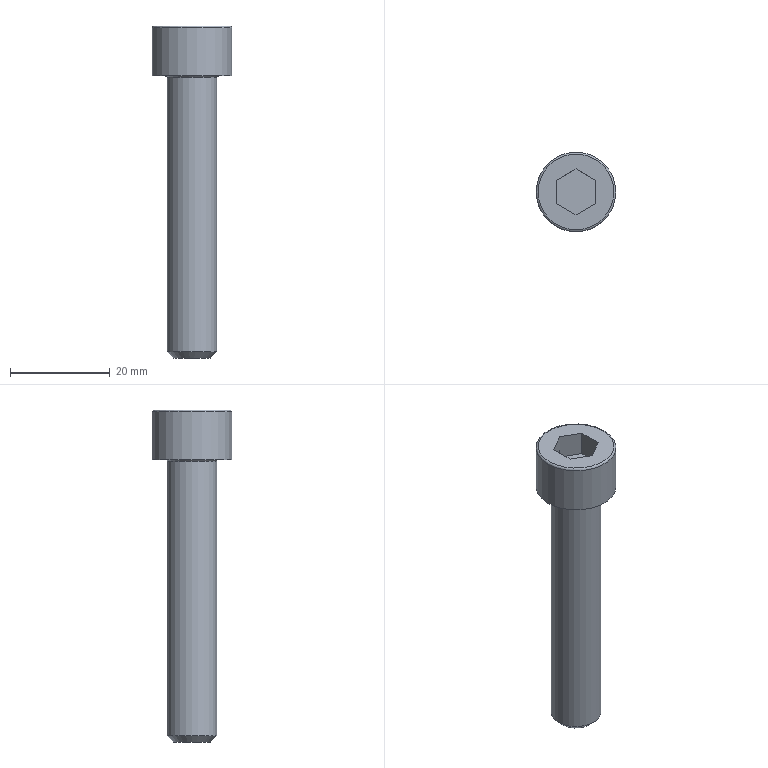Part | STEP file | solid 155 | 1 solid | 15 faces | box 16 x 16 x 66.6 mm | volume 6156 mm3 | plane 10 | cylinder 2 | torus 2 | cone 1 | commonest cylinder face diameters 10 x1 16 x1